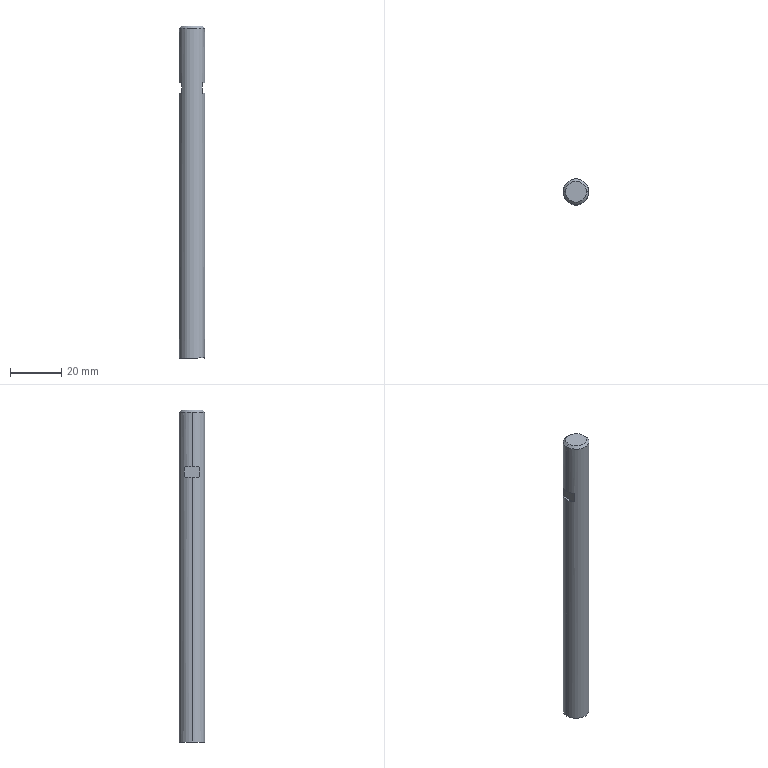Part | STEP file | fA_C85N25-100T(OUT) | 1 solid | 12 faces | box 10 x 10 x 129 mm | volume 10086 mm3 | plane 8 | cylinder 2 | cone 2 | commonest cylinder face diameters 10 x2
STEP:
#1=CARTESIAN_POINT('',(0.,0.,0.));
#2=DIRECTION('',(0.,0.,1.));
#3=DIRECTION('',(1.,0.,0.));
#4=AXIS2_PLACEMENT_3D('',#1,#2,#3);
#5=CARTESIAN_POINT('',(5.,0.,-1.));
#6=VERTEX_POINT('',#5);
#7=CARTESIAN_POINT('',(-5.,0.,-1.));
#8=VERTEX_POINT('',#7);
#9=CARTESIAN_POINT('',(0.,0.,-1.));
#10=DIRECTION('',(0.,0.,1.));
#11=DIRECTION('',(1.,0.,0.));
#12=AXIS2_PLACEMENT_3D('',#9,#10,#11);
#13=CIRCLE('',#12,5.);
#14=CARTESIAN_POINT('',(0.,0.,127.08));
#15=DIRECTION('',(0.,0.,1.));
#16=DIRECTION('',(1.,0.,0.));
#17=AXIS2_PLACEMENT_3D('',#14,#15,#16);
#18=CYLINDRICAL_SURFACE('',#17,5.);
#19=CARTESIAN_POINT('',(0.,-128.08));
#20=DIRECTION('',(1.,0.));
#21=VECTOR('',#20,1.);
#22=LINE('',#19,#21);
#23=(GEOMETRIC_REPRESENTATION_CONTEXT(2)PARAMETRIC_REPRESENTATION_CONTEXT()REPRESENTATION_CONTEXT('',''));
#24=DEFINITIONAL_REPRESENTATION('',(#22),#23);
#25=PCURVE('',#18,#24);
#26=CARTESIAN_POINT('',(5.06,5.,-1.));
#27=DIRECTION('',(0.,0.,-1.));
#28=DIRECTION('',(0.,1.,0.));
#29=AXIS2_PLACEMENT_3D('',#26,#27,#28);
#30=PLANE('',#29);
#31=CARTESIAN_POINT('',(-5.,-0.06));
#32=CARTESIAN_POINT('',(3.66,-0.06));
#33=CARTESIAN_POINT('',(-0.6699,-7.56));
#34=CARTESIAN_POINT('',(-5.,-15.06));
#35=CARTESIAN_POINT('',(-9.33,-7.56));
#36=CARTESIAN_POINT('',(-13.66,-0.06));
#37=CARTESIAN_POINT('',(-5.,-0.06));
#38=(BOUNDED_CURVE()B_SPLINE_CURVE(2,(#31,#32,#33,#34,#35,#36,#37),.UNSPECIFIED.,.T.,.F.)B_SPLINE_CURVE_WITH_KNOTS((1,2,2,2,2,1),(-2.094,0.,2.094,4.189,6.283,8.378),.UNSPECIFIED.)CURVE()GEOMETRIC_REPRESENTATION_ITEM()RATIONAL_B_SPLINE_CURVE((1.,0.5,1.,0.5,1.,0.5,1.))REPRESENTATION_ITEM(''));
#39=(GEOMETRIC_REPRESENTATION_CONTEXT(2)PARAMETRIC_REPRESENTATION_CONTEXT()REPRESENTATION_CONTEXT('',''));
#40=DEFINITIONAL_REPRESENTATION('',(#38),#39);
#41=PCURVE('',#30,#40);
#42=SURFACE_CURVE('',#13,(#25,#41),.PCURVE_S1.);
#43=EDGE_CURVE('',#6,#8,#42,.T.);
#44=ORIENTED_EDGE('',*,*,#43,.T.);
#45=CARTESIAN_POINT('',(-5.,0.,101.9));
#46=VERTEX_POINT('',#45);
#47=CARTESIAN_POINT('',(-5.,0.,127.08));
#48=DIRECTION('',(0.,0.,1.));
#49=VECTOR('',#48,1.);
#50=LINE('',#47,#49);
#51=CARTESIAN_POINT('',(3.142,0.));
#52=DIRECTION('',(0.,1.));
#53=VECTOR('',#52,1.);
#54=LINE('',#51,#53);
#55=(GEOMETRIC_REPRESENTATION_CONTEXT(2)PARAMETRIC_REPRESENTATION_CONTEXT()REPRESENTATION_CONTEXT('',''));
#56=DEFINITIONAL_REPRESENTATION('',(#54),#55);
#57=PCURVE('',#18,#56);
#58=CARTESIAN_POINT('',(0.,0.,127.08));
#59=DIRECTION('',(0.,0.,1.));
#60=DIRECTION('',(1.,0.,0.));
#61=AXIS2_PLACEMENT_3D('',#58,#59,#60);
#62=CYLINDRICAL_SURFACE('',#61,5.);
#63=CARTESIAN_POINT('',(3.142,0.));
#64=DIRECTION('',(0.,1.));
#65=VECTOR('',#64,1.);
#66=LINE('',#63,#65);
#67=(GEOMETRIC_REPRESENTATION_CONTEXT(2)PARAMETRIC_REPRESENTATION_CONTEXT()REPRESENTATION_CONTEXT('',''));
#68=DEFINITIONAL_REPRESENTATION('',(#66),#67);
#69=PCURVE('',#62,#68);
#70=SURFACE_CURVE('',#50,(#57,#69),.PCURVE_S1.);
#71=EDGE_CURVE('',#8,#46,#70,.T.);
#72=ORIENTED_EDGE('',*,*,#71,.T.);
#73=CARTESIAN_POINT('',(-4.,3.,101.9));
#74=VERTEX_POINT('',#73);
#75=CARTESIAN_POINT('',(0.,0.,101.9));
#76=DIRECTION('',(0.,0.,-1.));
#77=DIRECTION('',(1.,0.,0.));
#78=AXIS2_PLACEMENT_3D('',#75,#76,#77);
#79=CIRCLE('',#78,5.);
#80=CARTESIAN_POINT('',(6.283,-25.18));
#81=DIRECTION('',(-1.,0.));
#82=VECTOR('',#81,1.);
#83=LINE('',#80,#82);
#84=(GEOMETRIC_REPRESENTATION_CONTEXT(2)PARAMETRIC_REPRESENTATION_CONTEXT()REPRESENTATION_CONTEXT('',''));
#85=DEFINITIONAL_REPRESENTATION('',(#83),#84);
#86=PCURVE('',#18,#85);
#87=CARTESIAN_POINT('',(-5.006,-3.036,101.9));
#88=DIRECTION('',(0.,0.,1.));
#89=DIRECTION('',(1.,0.,0.));
#90=AXIS2_PLACEMENT_3D('',#87,#88,#89);
#91=PLANE('',#90);
#92=CARTESIAN_POINT('',(10.006,3.036));
#93=CARTESIAN_POINT('',(10.006,-5.624));
#94=CARTESIAN_POINT('',(2.506,-1.294));
#95=CARTESIAN_POINT('',(-4.994,3.036));
#96=CARTESIAN_POINT('',(2.506,7.366));
#97=CARTESIAN_POINT('',(10.006,11.696));
#98=CARTESIAN_POINT('',(10.006,3.036));
#99=(BOUNDED_CURVE()B_SPLINE_CURVE(2,(#92,#93,#94,#95,#96,#97,#98),.UNSPECIFIED.,.T.,.F.)B_SPLINE_CURVE_WITH_KNOTS((1,2,2,2,2,1),(-2.094,0.,2.094,4.189,6.283,8.378),.UNSPECIFIED.)CURVE()GEOMETRIC_REPRESENTATION_ITEM()RATIONAL_B_SPLINE_CURVE((1.,0.5,1.,0.5,1.,0.5,1.))REPRESENTATION_ITEM(''));
#100=(GEOMETRIC_REPRESENTATION_CONTEXT(2)PARAMETRIC_REPRESENTATION_CONTEXT()REPRESENTATION_CONTEXT('',''));
#101=DEFINITIONAL_REPRESENTATION('',(#99),#100);
#102=PCURVE('',#91,#101);
#103=SURFACE_CURVE('',#79,(#86,#102),.PCURVE_S1.);
#104=EDGE_CURVE('',#46,#74,#103,.T.);
#105=ORIENTED_EDGE('',*,*,#104,.T.);
#106=CARTESIAN_POINT('',(-4.,3.,105.9));
#107=VERTEX_POINT('',#106);
#108=CARTESIAN_POINT('',(-4.,3.,127.08));
#109=DIRECTION('',(0.,0.,1.));
#110=VECTOR('',#109,1.);
#111=LINE('',#108,#110);
#112=CARTESIAN_POINT('',(2.498,0.));
#113=DIRECTION('',(0.,1.));
#114=VECTOR('',#113,1.);
#115=LINE('',#112,#114);
#116=(GEOMETRIC_REPRESENTATION_CONTEXT(2)PARAMETRIC_REPRESENTATION_CONTEXT()REPRESENTATION_CONTEXT('',''));
#117=DEFINITIONAL_REPRESENTATION('',(#115),#116);
#118=PCURVE('',#18,#117);
#119=CARTESIAN_POINT('',(-4.,-3.,105.9));
#120=DIRECTION('',(-1.,0.,0.));
#121=DIRECTION('',(0.,0.,1.));
#122=AXIS2_PLACEMENT_3D('',#119,#120,#121);
#123=PLANE('',#122);
#124=CARTESIAN_POINT('',(21.18,6.));
#125=DIRECTION('',(1.,0.));
#126=VECTOR('',#125,1.);
#127=LINE('',#124,#126);
#128=(GEOMETRIC_REPRESENTATION_CONTEXT(2)PARAMETRIC_REPRESENTATION_CONTEXT()REPRESENTATION_CONTEXT('',''));
#129=DEFINITIONAL_REPRESENTATION('',(#127),#128);
#130=PCURVE('',#123,#129);
#131=SURFACE_CURVE('',#111,(#118,#130),.PCURVE_S1.);
#132=EDGE_CURVE('',#74,#107,#131,.T.);
#133=ORIENTED_EDGE('',*,*,#132,.T.);
#134=CARTESIAN_POINT('',(-5.,0.,105.9));
#135=VERTEX_POINT('',#134);
#136=CARTESIAN_POINT('',(0.,0.,105.9));
#137=DIRECTION('',(0.,0.,1.));
#138=DIRECTION('',(1.,0.,0.));
#139=AXIS2_PLACEMENT_3D('',#136,#137,#138);
#140=CIRCLE('',#139,5.);
#141=CARTESIAN_POINT('',(0.,-21.18));
#142=DIRECTION('',(1.,0.));
#143=VECTOR('',#142,1.);
#144=LINE('',#141,#143);
#145=(GEOMETRIC_REPRESENTATION_CONTEXT(2)PARAMETRIC_REPRESENTATION_CONTEXT()REPRESENTATION_CONTEXT('',''));
#146=DEFINITIONAL_REPRESENTATION('',(#144),#145);
#147=PCURVE('',#18,#146);
#148=CARTESIAN_POINT('',(-4.,-3.036,105.9));
#149=DIRECTION('',(0.,0.,-1.));
#150=DIRECTION('',(-1.,0.,0.));
#151=AXIS2_PLACEMENT_3D('',#148,#149,#150);
#152=PLANE('',#151);
#153=CARTESIAN_POINT('',(-9.,3.036));
#154=CARTESIAN_POINT('',(-9.,11.696));
#155=CARTESIAN_POINT('',(-1.5,7.366));
#156=CARTESIAN_POINT('',(6.,3.036));
#157=CARTESIAN_POINT('',(-1.5,-1.294));
#158=CARTESIAN_POINT('',(-9.,-5.624));
#159=CARTESIAN_POINT('',(-9.,3.036));
#160=(BOUNDED_CURVE()B_SPLINE_CURVE(2,(#153,#154,#155,#156,#157,#158,#159),.UNSPECIFIED.,.T.,.F.)B_SPLINE_CURVE_WITH_KNOTS((1,2,2,2,2,1),(-2.094,0.,2.094,4.189,6.283,8.378),.UNSPECIFIED.)CURVE()GEOMETRIC_REPRESENTATION_ITEM()RATIONAL_B_SPLINE_CURVE((1.,0.5,1.,0.5,1.,0.5,1.))REPRESENTATION_ITEM(''));
#161=(GEOMETRIC_REPRESENTATION_CONTEXT(2)PARAMETRIC_REPRESENTATION_CONTEXT()REPRESENTATION_CONTEXT('',''));
#162=DEFINITIONAL_REPRESENTATION('',(#160),#161);
#163=PCURVE('',#152,#162);
#164=SURFACE_CURVE('',#140,(#147,#163),.PCURVE_S1.);
#165=EDGE_CURVE('',#107,#135,#164,.T.);
#166=ORIENTED_EDGE('',*,*,#165,.T.);
#167=CARTESIAN_POINT('',(-5.,0.,127.08));
#168=VERTEX_POINT('',#167);
#169=CARTESIAN_POINT('',(-5.,0.,127.08));
#170=DIRECTION('',(0.,0.,1.));
#171=VECTOR('',#170,1.);
#172=LINE('',#169,#171);
#173=CARTESIAN_POINT('',(3.142,0.));
#174=DIRECTION('',(0.,1.));
#175=VECTOR('',#174,1.);
#176=LINE('',#173,#175);
#177=(GEOMETRIC_REPRESENTATION_CONTEXT(2)PARAMETRIC_REPRESENTATION_CONTEXT()REPRESENTATION_CONTEXT('',''));
#178=DEFINITIONAL_REPRESENTATION('',(#176),#177);
#179=PCURVE('',#18,#178);
#180=CARTESIAN_POINT('',(3.142,0.));
#181=DIRECTION('',(0.,1.));
#182=VECTOR('',#181,1.);
#183=LINE('',#180,#182);
#184=(GEOMETRIC_REPRESENTATION_CONTEXT(2)PARAMETRIC_REPRESENTATION_CONTEXT()REPRESENTATION_CONTEXT('',''));
#185=DEFINITIONAL_REPRESENTATION('',(#183),#184);
#186=PCURVE('',#62,#185);
#187=SURFACE_CURVE('',#172,(#179,#186),.PCURVE_S1.);
#188=EDGE_CURVE('',#135,#168,#187,.T.);
#189=ORIENTED_EDGE('',*,*,#188,.T.);
#190=CARTESIAN_POINT('',(5.,0.,127.08));
#191=VERTEX_POINT('',#190);
#192=CARTESIAN_POINT('',(0.,0.,127.08));
#193=DIRECTION('',(0.,0.,-1.));
#194=DIRECTION('',(1.,0.,0.));
#195=AXIS2_PLACEMENT_3D('',#192,#193,#194);
#196=CIRCLE('',#195,5.);
#197=CARTESIAN_POINT('',(6.283,0.));
#198=DIRECTION('',(-1.,0.));
#199=VECTOR('',#198,1.);
#200=LINE('',#197,#199);
#201=(GEOMETRIC_REPRESENTATION_CONTEXT(2)PARAMETRIC_REPRESENTATION_CONTEXT()REPRESENTATION_CONTEXT('',''));
#202=DEFINITIONAL_REPRESENTATION('',(#200),#201);
#203=PCURVE('',#18,#202);
#204=CARTESIAN_POINT('',(0.,0.,127.08));
#205=DIRECTION('',(0.,0.,-1.));
#206=DIRECTION('',(-1.,0.,0.));
#207=AXIS2_PLACEMENT_3D('',#204,#205,#206);
#208=CONICAL_SURFACE('',#207,5.,0.7854);
#209=CARTESIAN_POINT('',(-3.142,0.));
#210=DIRECTION('',(1.,0.));
#211=VECTOR('',#210,1.);
#212=LINE('',#209,#211);
#213=(GEOMETRIC_REPRESENTATION_CONTEXT(2)PARAMETRIC_REPRESENTATION_CONTEXT()REPRESENTATION_CONTEXT('',''));
#214=DEFINITIONAL_REPRESENTATION('',(#212),#213);
#215=PCURVE('',#208,#214);
#216=SURFACE_CURVE('',#196,(#203,#215),.PCURVE_S1.);
#217=EDGE_CURVE('',#168,#191,#216,.T.);
#218=ORIENTED_EDGE('',*,*,#217,.T.);
#219=CARTESIAN_POINT('',(5.,0.,105.9));
#220=VERTEX_POINT('',#219);
#221=CARTESIAN_POINT('',(5.,0.,127.08));
#222=DIRECTION('',(0.,0.,1.));
#223=VECTOR('',#222,1.);
#224=LINE('',#221,#223);
#225=CARTESIAN_POINT('',(0.,0.));
#226=DIRECTION('',(0.,1.));
#227=VECTOR('',#226,1.);
#228=LINE('',#225,#227);
#229=(GEOMETRIC_REPRESENTATION_CONTEXT(2)PARAMETRIC_REPRESENTATION_CONTEXT()REPRESENTATION_CONTEXT('',''));
#230=DEFINITIONAL_REPRESENTATION('',(#228),#229);
#231=PCURVE('',#18,#230);
#232=CARTESIAN_POINT('',(6.283,0.));
#233=DIRECTION('',(0.,1.));
#234=VECTOR('',#233,1.);
#235=LINE('',#232,#234);
#236=(GEOMETRIC_REPRESENTATION_CONTEXT(2)PARAMETRIC_REPRESENTATION_CONTEXT()REPRESENTATION_CONTEXT('',''));
#237=DEFINITIONAL_REPRESENTATION('',(#235),#236);
#238=PCURVE('',#62,#237);
#239=SURFACE_CURVE('',#224,(#231,#238),.PCURVE_S1.);
#240=EDGE_CURVE('',#220,#191,#239,.T.);
#241=ORIENTED_EDGE('',*,*,#240,.F.);
#242=CARTESIAN_POINT('',(4.,3.,105.9));
#243=VERTEX_POINT('',#242);
#244=CARTESIAN_POINT('',(0.,0.,105.9));
#245=DIRECTION('',(0.,0.,1.));
#246=DIRECTION('',(1.,0.,0.));
#247=AXIS2_PLACEMENT_3D('',#244,#245,#246);
#248=CIRCLE('',#247,5.);
#249=CARTESIAN_POINT('',(0.,-21.18));
#250=DIRECTION('',(1.,0.));
#251=VECTOR('',#250,1.);
#252=LINE('',#249,#251);
#253=(GEOMETRIC_REPRESENTATION_CONTEXT(2)PARAMETRIC_REPRESENTATION_CONTEXT()REPRESENTATION_CONTEXT('',''));
#254=DEFINITIONAL_REPRESENTATION('',(#252),#253);
#255=PCURVE('',#18,#254);
#256=CARTESIAN_POINT('',(5.006,-3.036,105.9));
#257=DIRECTION('',(0.,0.,-1.));
#258=DIRECTION('',(-1.,0.,0.));
#259=AXIS2_PLACEMENT_3D('',#256,#257,#258);
#260=PLANE('',#259);
#261=CARTESIAN_POINT('',(0.006,3.036));
#262=CARTESIAN_POINT('',(0.006,11.696));
#263=CARTESIAN_POINT('',(7.506,7.366));
#264=CARTESIAN_POINT('',(15.006,3.036));
#265=CARTESIAN_POINT('',(7.506,-1.294));
#266=CARTESIAN_POINT('',(0.006,-5.624));
#267=CARTESIAN_POINT('',(0.006,3.036));
#268=(BOUNDED_CURVE()B_SPLINE_CURVE(2,(#261,#262,#263,#264,#265,#266,#267),.UNSPECIFIED.,.T.,.F.)B_SPLINE_CURVE_WITH_KNOTS((1,2,2,2,2,1),(-2.094,0.,2.094,4.189,6.283,8.378),.UNSPECIFIED.)CURVE()GEOMETRIC_REPRESENTATION_ITEM()RATIONAL_B_SPLINE_CURVE((1.,0.5,1.,0.5,1.,0.5,1.))REPRESENTATION_ITEM(''));
#269=(GEOMETRIC_REPRESENTATION_CONTEXT(2)PARAMETRIC_REPRESENTATION_CONTEXT()REPRESENTATION_CONTEXT('',''));
#270=DEFINITIONAL_REPRESENTATION('',(#268),#269);
#271=PCURVE('',#260,#270);
#272=SURFACE_CURVE('',#248,(#255,#271),.PCURVE_S1.);
#273=EDGE_CURVE('',#220,#243,#272,.T.);
#274=ORIENTED_EDGE('',*,*,#273,.T.);
#275=CARTESIAN_POINT('',(4.,3.,101.9));
#276=VERTEX_POINT('',#275);
#277=CARTESIAN_POINT('',(4.,3.,127.08));
#278=DIRECTION('',(0.,0.,-1.));
#279=VECTOR('',#278,1.);
#280=LINE('',#277,#279);
#281=CARTESIAN_POINT('',(0.6435,0.));
#282=DIRECTION('',(0.,-1.));
#283=VECTOR('',#282,1.);
#284=LINE('',#281,#283);
#285=(GEOMETRIC_REPRESENTATION_CONTEXT(2)PARAMETRIC_REPRESENTATION_CONTEXT()REPRESENTATION_CONTEXT('',''));
#286=DEFINITIONAL_REPRESENTATION('',(#284),#285);
#287=PCURVE('',#18,#286);
#288=CARTESIAN_POINT('',(4.,3.,105.9));
#289=DIRECTION('',(1.,0.,0.));
#290=DIRECTION('',(0.,0.,-1.));
#291=AXIS2_PLACEMENT_3D('',#288,#289,#290);
#292=PLANE('',#291);
#293=CARTESIAN_POINT('',(-21.18,0.));
#294=DIRECTION('',(1.,0.));
#295=VECTOR('',#294,1.);
#296=LINE('',#293,#295);
#297=(GEOMETRIC_REPRESENTATION_CONTEXT(2)PARAMETRIC_REPRESENTATION_CONTEXT()REPRESENTATION_CONTEXT('',''));
#298=DEFINITIONAL_REPRESENTATION('',(#296),#297);
#299=PCURVE('',#292,#298);
#300=SURFACE_CURVE('',#280,(#287,#299),.PCURVE_S1.);
#301=EDGE_CURVE('',#243,#276,#300,.T.);
#302=ORIENTED_EDGE('',*,*,#301,.T.);
#303=CARTESIAN_POINT('',(5.,0.,101.9));
#304=VERTEX_POINT('',#303);
#305=CARTESIAN_POINT('',(0.,0.,101.9));
#306=DIRECTION('',(0.,0.,-1.));
#307=DIRECTION('',(1.,0.,0.));
#308=AXIS2_PLACEMENT_3D('',#305,#306,#307);
#309=CIRCLE('',#308,5.);
#310=CARTESIAN_POINT('',(6.283,-25.18));
#311=DIRECTION('',(-1.,0.));
#312=VECTOR('',#311,1.);
#313=LINE('',#310,#312);
#314=(GEOMETRIC_REPRESENTATION_CONTEXT(2)PARAMETRIC_REPRESENTATION_CONTEXT()REPRESENTATION_CONTEXT('',''));
#315=DEFINITIONAL_REPRESENTATION('',(#313),#314);
#316=PCURVE('',#18,#315);
#317=CARTESIAN_POINT('',(4.,-3.036,101.9));
#318=DIRECTION('',(0.,0.,1.));
#319=DIRECTION('',(1.,0.,0.));
#320=AXIS2_PLACEMENT_3D('',#317,#318,#319);
#321=PLANE('',#320);
#322=CARTESIAN_POINT('',(1.,3.036));
#323=CARTESIAN_POINT('',(1.,-5.624));
#324=CARTESIAN_POINT('',(-6.5,-1.294));
#325=CARTESIAN_POINT('',(-14.,3.036));
#326=CARTESIAN_POINT('',(-6.5,7.366));
#327=CARTESIAN_POINT('',(1.,11.696));
#328=CARTESIAN_POINT('',(1.,3.036));
#329=(BOUNDED_CURVE()B_SPLINE_CURVE(2,(#322,#323,#324,#325,#326,#327,#328),.UNSPECIFIED.,.T.,.F.)B_SPLINE_CURVE_WITH_KNOTS((1,2,2,2,2,1),(-2.094,0.,2.094,4.189,6.283,8.378),.UNSPECIFIED.)CURVE()GEOMETRIC_REPRESENTATION_ITEM()RATIONAL_B_SPLINE_CURVE((1.,0.5,1.,0.5,1.,0.5,1.))REPRESENTATION_ITEM(''));
#330=(GEOMETRIC_REPRESENTATION_CONTEXT(2)PARAMETRIC_REPRESENTATION_CONTEXT()REPRESENTATION_CONTEXT('',''));
#331=DEFINITIONAL_REPRESENTATION('',(#329),#330);
#332=PCURVE('',#321,#331);
#333=SURFACE_CURVE('',#309,(#316,#332),.PCURVE_S1.);
#334=EDGE_CURVE('',#276,#304,#333,.T.);
#335=ORIENTED_EDGE('',*,*,#334,.T.);
#336=CARTESIAN_POINT('',(5.,0.,127.08));
#337=DIRECTION('',(0.,0.,1.));
#338=VECTOR('',#337,1.);
#339=LINE('',#336,#338);
#340=CARTESIAN_POINT('',(0.,0.));
#341=DIRECTION('',(0.,1.));
#342=VECTOR('',#341,1.);
#343=LINE('',#340,#342);
#344=(GEOMETRIC_REPRESENTATION_CONTEXT(2)PARAMETRIC_REPRESENTATION_CONTEXT()REPRESENTATION_CONTEXT('',''));
#345=DEFINITIONAL_REPRESENTATION('',(#343),#344);
#346=PCURVE('',#18,#345);
#347=CARTESIAN_POINT('',(6.283,0.));
#348=DIRECTION('',(0.,1.));
#349=VECTOR('',#348,1.);
#350=LINE('',#347,#349);
#351=(GEOMETRIC_REPRESENTATION_CONTEXT(2)PARAMETRIC_REPRESENTATION_CONTEXT()REPRESENTATION_CONTEXT('',''));
#352=DEFINITIONAL_REPRESENTATION('',(#350),#351);
#353=PCURVE('',#62,#352);
#354=SURFACE_CURVE('',#339,(#346,#353),.PCURVE_S1.);
#355=EDGE_CURVE('',#6,#304,#354,.T.);
#356=ORIENTED_EDGE('',*,*,#355,.F.);
#357=EDGE_LOOP('',(#44,#72,#105,#133,#166,#189,#218,#241,#274,#302,#335,#356));
#358=FACE_BOUND('',#357,.T.);
#359=ADVANCED_FACE('',(#358),#18,.T.);
#360=CARTESIAN_POINT('',(-4.08,0.,128.));
#361=VERTEX_POINT('',#360);
#362=CARTESIAN_POINT('',(4.08,0.,128.));
#363=VERTEX_POINT('',#362);
#364=CARTESIAN_POINT('',(0.,0.,128.));
#365=DIRECTION('',(0.,0.,-1.));
#366=DIRECTION('',(-1.,0.,0.));
#367=AXIS2_PLACEMENT_3D('',#364,#365,#366);
#368=CIRCLE('',#367,4.08);
#369=CARTESIAN_POINT('',(0.,-0.92));
#370=DIRECTION('',(1.,0.));
#371=VECTOR('',#370,1.);
#372=LINE('',#369,#371);
#373=(GEOMETRIC_REPRESENTATION_CONTEXT(2)PARAMETRIC_REPRESENTATION_CONTEXT()REPRESENTATION_CONTEXT('',''));
#374=DEFINITIONAL_REPRESENTATION('',(#372),#373);
#375=PCURVE('',#208,#374);
#376=CARTESIAN_POINT('',(4.129,-4.08,128.));
#377=DIRECTION('',(0.,0.,1.));
#378=DIRECTION('',(1.,0.,0.));
#379=AXIS2_PLACEMENT_3D('',#376,#377,#378);
#380=PLANE('',#379);
#381=CARTESIAN_POINT('',(-8.209,4.08));
#382=CARTESIAN_POINT('',(-8.209,11.147));
#383=CARTESIAN_POINT('',(-2.089,7.613));
#384=CARTESIAN_POINT('',(4.031,4.08));
#385=CARTESIAN_POINT('',(-2.089,0.5466));
#386=CARTESIAN_POINT('',(-8.209,-2.987));
#387=CARTESIAN_POINT('',(-8.209,4.08));
#388=(BOUNDED_CURVE()B_SPLINE_CURVE(2,(#381,#382,#383,#384,#385,#386,#387),.UNSPECIFIED.,.T.,.F.)B_SPLINE_CURVE_WITH_KNOTS((1,2,2,2,2,1),(-2.094,0.,2.094,4.189,6.283,8.378),.UNSPECIFIED.)CURVE()GEOMETRIC_REPRESENTATION_ITEM()RATIONAL_B_SPLINE_CURVE((1.,0.5,1.,0.5,1.,0.5,1.))REPRESENTATION_ITEM(''));
#389=(GEOMETRIC_REPRESENTATION_CONTEXT(2)PARAMETRIC_REPRESENTATION_CONTEXT()REPRESENTATION_CONTEXT('',''));
#390=DEFINITIONAL_REPRESENTATION('',(#388),#389);
#391=PCURVE('',#380,#390);
#392=SURFACE_CURVE('',#368,(#375,#391),.PCURVE_S1.);
#393=EDGE_CURVE('',#361,#363,#392,.T.);
#394=ORIENTED_EDGE('',*,*,#393,.T.);
#395=CARTESIAN_POINT('',(5.,0.,127.08));
#396=DIRECTION('',(0.7071,0.,-0.7071));
#397=VECTOR('',#396,1.);
#398=LINE('',#395,#397);
#399=CARTESIAN_POINT('',(3.142,0.));
#400=DIRECTION('',(0.,1.));
#401=VECTOR('',#400,1.);
#402=LINE('',#399,#401);
#403=(GEOMETRIC_REPRESENTATION_CONTEXT(2)PARAMETRIC_REPRESENTATION_CONTEXT()REPRESENTATION_CONTEXT('',''));
#404=DEFINITIONAL_REPRESENTATION('',(#402),#403);
#405=PCURVE('',#208,#404);
#406=CARTESIAN_POINT('',(0.,0.,127.08));
#407=DIRECTION('',(0.,0.,-1.));
#408=DIRECTION('',(-1.,0.,0.));
#409=AXIS2_PLACEMENT_3D('',#406,#407,#408);
#410=CONICAL_SURFACE('',#409,5.,0.7854);
#411=CARTESIAN_POINT('',(3.142,0.));
#412=DIRECTION('',(0.,1.));
#413=VECTOR('',#412,1.);
#414=LINE('',#411,#413);
#415=(GEOMETRIC_REPRESENTATION_CONTEXT(2)PARAMETRIC_REPRESENTATION_CONTEXT()REPRESENTATION_CONTEXT('',''));
#416=DEFINITIONAL_REPRESENTATION('',(#414),#415);
#417=PCURVE('',#410,#416);
#418=SURFACE_CURVE('',#398,(#405,#417),.PCURVE_S1.);
#419=EDGE_CURVE('',#363,#191,#418,.T.);
#420=ORIENTED_EDGE('',*,*,#419,.T.);
#421=ORIENTED_EDGE('',*,*,#217,.F.);
#422=CARTESIAN_POINT('',(-5.,0.,127.08));
#423=DIRECTION('',(-0.7071,0.,-0.7071));
#424=VECTOR('',#423,1.);
#425=LINE('',#422,#424);
#426=CARTESIAN_POINT('',(0.,0.));
#427=DIRECTION('',(0.,1.));
#428=VECTOR('',#427,1.);
#429=LINE('',#426,#428);
#430=(GEOMETRIC_REPRESENTATION_CONTEXT(2)PARAMETRIC_REPRESENTATION_CONTEXT()REPRESENTATION_CONTEXT('',''));
#431=DEFINITIONAL_REPRESENTATION('',(#429),#430);
#432=PCURVE('',#208,#431);
#433=CARTESIAN_POINT('',(6.283,0.));
#434=DIRECTION('',(0.,1.));
#435=VECTOR('',#434,1.);
#436=LINE('',#433,#435);
#437=(GEOMETRIC_REPRESENTATION_CONTEXT(2)PARAMETRIC_REPRESENTATION_CONTEXT()REPRESENTATION_CONTEXT('',''));
#438=DEFINITIONAL_REPRESENTATION('',(#436),#437);
#439=PCURVE('',#410,#438);
#440=SURFACE_CURVE('',#425,(#432,#439),.PCURVE_S1.);
#441=EDGE_CURVE('',#361,#168,#440,.T.);
#442=ORIENTED_EDGE('',*,*,#441,.F.);
#443=EDGE_LOOP('',(#394,#420,#421,#442));
#444=FACE_BOUND('',#443,.T.);
#445=ADVANCED_FACE('',(#444),#208,.T.);
#446=ORIENTED_EDGE('',*,*,#71,.F.);
#447=CARTESIAN_POINT('',(0.,0.,-1.));
#448=DIRECTION('',(0.,0.,1.));
#449=DIRECTION('',(1.,0.,0.));
#450=AXIS2_PLACEMENT_3D('',#447,#448,#449);
#451=CIRCLE('',#450,5.);
#452=CARTESIAN_POINT('',(0.,-128.08));
#453=DIRECTION('',(1.,0.));
#454=VECTOR('',#453,1.);
#455=LINE('',#452,#454);
#456=(GEOMETRIC_REPRESENTATION_CONTEXT(2)PARAMETRIC_REPRESENTATION_CONTEXT()REPRESENTATION_CONTEXT('',''));
#457=DEFINITIONAL_REPRESENTATION('',(#455),#456);
#458=PCURVE('',#62,#457);
#459=CARTESIAN_POINT('',(-5.,-0.06));
#460=CARTESIAN_POINT('',(3.66,-0.06));
#461=CARTESIAN_POINT('',(-0.6699,-7.56));
#462=CARTESIAN_POINT('',(-5.,-15.06));
#463=CARTESIAN_POINT('',(-9.33,-7.56));
#464=CARTESIAN_POINT('',(-13.66,-0.06));
#465=CARTESIAN_POINT('',(-5.,-0.06));
#466=(BOUNDED_CURVE()B_SPLINE_CURVE(2,(#459,#460,#461,#462,#463,#464,#465),.UNSPECIFIED.,.T.,.F.)B_SPLINE_CURVE_WITH_KNOTS((1,2,2,2,2,1),(-2.094,0.,2.094,4.189,6.283,8.378),.UNSPECIFIED.)CURVE()GEOMETRIC_REPRESENTATION_ITEM()RATIONAL_B_SPLINE_CURVE((1.,0.5,1.,0.5,1.,0.5,1.))REPRESENTATION_ITEM(''));
#467=(GEOMETRIC_REPRESENTATION_CONTEXT(2)PARAMETRIC_REPRESENTATION_CONTEXT()REPRESENTATION_CONTEXT('',''));
#468=DEFINITIONAL_REPRESENTATION('',(#466),#467);
#469=PCURVE('',#30,#468);
#470=SURFACE_CURVE('',#451,(#458,#469),.PCURVE_S1.);
#471=EDGE_CURVE('',#8,#6,#470,.T.);
#472=ORIENTED_EDGE('',*,*,#471,.T.);
#473=ORIENTED_EDGE('',*,*,#355,.T.);
#474=CARTESIAN_POINT('',(4.,-3.,101.9));
#475=VERTEX_POINT('',#474);
#476=CARTESIAN_POINT('',(0.,0.,101.9));
#477=DIRECTION('',(0.,0.,-1.));
#478=DIRECTION('',(1.,0.,0.));
#479=AXIS2_PLACEMENT_3D('',#476,#477,#478);
#480=CIRCLE('',#479,5.);
#481=CARTESIAN_POINT('',(6.283,-25.18));
#482=DIRECTION('',(-1.,0.));
#483=VECTOR('',#482,1.);
#484=LINE('',#481,#483);
#485=(GEOMETRIC_REPRESENTATION_CONTEXT(2)PARAMETRIC_REPRESENTATION_CONTEXT()REPRESENTATION_CONTEXT('',''));
#486=DEFINITIONAL_REPRESENTATION('',(#484),#485);
#487=PCURVE('',#62,#486);
#488=CARTESIAN_POINT('',(1.,3.036));
#489=CARTESIAN_POINT('',(1.,-5.624));
#490=CARTESIAN_POINT('',(-6.5,-1.294));
#491=CARTESIAN_POINT('',(-14.,3.036));
#492=CARTESIAN_POINT('',(-6.5,7.366));
#493=CARTESIAN_POINT('',(1.,11.696));
#494=CARTESIAN_POINT('',(1.,3.036));
#495=(BOUNDED_CURVE()B_SPLINE_CURVE(2,(#488,#489,#490,#491,#492,#493,#494),.UNSPECIFIED.,.T.,.F.)B_SPLINE_CURVE_WITH_KNOTS((1,2,2,2,2,1),(-2.094,0.,2.094,4.189,6.283,8.378),.UNSPECIFIED.)CURVE()GEOMETRIC_REPRESENTATION_ITEM()RATIONAL_B_SPLINE_CURVE((1.,0.5,1.,0.5,1.,0.5,1.))REPRESENTATION_ITEM(''));
#496=(GEOMETRIC_REPRESENTATION_CONTEXT(2)PARAMETRIC_REPRESENTATION_CONTEXT()REPRESENTATION_CONTEXT('',''));
#497=DEFINITIONAL_REPRESENTATION('',(#495),#496);
#498=PCURVE('',#321,#497);
#499=SURFACE_CURVE('',#480,(#487,#498),.PCURVE_S1.);
#500=EDGE_CURVE('',#304,#475,#499,.T.);
#501=ORIENTED_EDGE('',*,*,#500,.T.);
#502=CARTESIAN_POINT('',(4.,-3.,105.9));
#503=VERTEX_POINT('',#502);
#504=CARTESIAN_POINT('',(4.,-3.,127.08));
#505=DIRECTION('',(0.,0.,1.));
#506=VECTOR('',#505,1.);
#507=LINE('',#504,#506);
#508=CARTESIAN_POINT('',(5.64,0.));
#509=DIRECTION('',(0.,1.));
#510=VECTOR('',#509,1.);
#511=LINE('',#508,#510);
#512=(GEOMETRIC_REPRESENTATION_CONTEXT(2)PARAMETRIC_REPRESENTATION_CONTEXT()REPRESENTATION_CONTEXT('',''));
#513=DEFINITIONAL_REPRESENTATION('',(#511),#512);
#514=PCURVE('',#62,#513);
#515=CARTESIAN_POINT('',(-21.18,-6.));
#516=DIRECTION('',(-1.,0.));
#517=VECTOR('',#516,1.);
#518=LINE('',#515,#517);
#519=(GEOMETRIC_REPRESENTATION_CONTEXT(2)PARAMETRIC_REPRESENTATION_CONTEXT()REPRESENTATION_CONTEXT('',''));
#520=DEFINITIONAL_REPRESENTATION('',(#518),#519);
#521=PCURVE('',#292,#520);
#522=SURFACE_CURVE('',#507,(#514,#521),.PCURVE_S1.);
#523=EDGE_CURVE('',#475,#503,#522,.T.);
#524=ORIENTED_EDGE('',*,*,#523,.T.);
#525=CARTESIAN_POINT('',(0.,0.,105.9));
#526=DIRECTION('',(0.,0.,1.));
#527=DIRECTION('',(1.,0.,0.));
#528=AXIS2_PLACEMENT_3D('',#525,#526,#527);
#529=CIRCLE('',#528,5.);
#530=CARTESIAN_POINT('',(0.,-21.18));
#531=DIRECTION('',(1.,0.));
#532=VECTOR('',#531,1.);
#533=LINE('',#530,#532);
#534=(GEOMETRIC_REPRESENTATION_CONTEXT(2)PARAMETRIC_REPRESENTATION_CONTEXT()REPRESENTATION_CONTEXT('',''));
#535=DEFINITIONAL_REPRESENTATION('',(#533),#534);
#536=PCURVE('',#62,#535);
#537=CARTESIAN_POINT('',(0.006,3.036));
#538=CARTESIAN_POINT('',(0.006,11.696));
#539=CARTESIAN_POINT('',(7.506,7.366));
#540=CARTESIAN_POINT('',(15.006,3.036));
#541=CARTESIAN_POINT('',(7.506,-1.294));
#542=CARTESIAN_POINT('',(0.006,-5.624));
#543=CARTESIAN_POINT('',(0.006,3.036));
#544=(BOUNDED_CURVE()B_SPLINE_CURVE(2,(#537,#538,#539,#540,#541,#542,#543),.UNSPECIFIED.,.T.,.F.)B_SPLINE_CURVE_WITH_KNOTS((1,2,2,2,2,1),(-2.094,0.,2.094,4.189,6.283,8.378),.UNSPECIFIED.)CURVE()GEOMETRIC_REPRESENTATION_ITEM()RATIONAL_B_SPLINE_CURVE((1.,0.5,1.,0.5,1.,0.5,1.))REPRESENTATION_ITEM(''));
#545=(GEOMETRIC_REPRESENTATION_CONTEXT(2)PARAMETRIC_REPRESENTATION_CONTEXT()REPRESENTATION_CONTEXT('',''));
#546=DEFINITIONAL_REPRESENTATION('',(#544),#545);
#547=PCURVE('',#260,#546);
#548=SURFACE_CURVE('',#529,(#536,#547),.PCURVE_S1.);
#549=EDGE_CURVE('',#503,#220,#548,.T.);
#550=ORIENTED_EDGE('',*,*,#549,.T.);
#551=ORIENTED_EDGE('',*,*,#240,.T.);
#552=CARTESIAN_POINT('',(0.,0.,127.08));
#553=DIRECTION('',(0.,0.,-1.));
#554=DIRECTION('',(1.,0.,0.));
#555=AXIS2_PLACEMENT_3D('',#552,#553,#554);
#556=CIRCLE('',#555,5.);
#557=CARTESIAN_POINT('',(6.283,0.));
#558=DIRECTION('',(-1.,0.));
#559=VECTOR('',#558,1.);
#560=LINE('',#557,#559);
#561=(GEOMETRIC_REPRESENTATION_CONTEXT(2)PARAMETRIC_REPRESENTATION_CONTEXT()REPRESENTATION_CONTEXT('',''));
#562=DEFINITIONAL_REPRESENTATION('',(#560),#561);
#563=PCURVE('',#62,#562);
#564=CARTESIAN_POINT('',(3.142,0.));
#565=DIRECTION('',(1.,0.));
#566=VECTOR('',#565,1.);
#567=LINE('',#564,#566);
#568=(GEOMETRIC_REPRESENTATION_CONTEXT(2)PARAMETRIC_REPRESENTATION_CONTEXT()REPRESENTATION_CONTEXT('',''));
#569=DEFINITIONAL_REPRESENTATION('',(#567),#568);
#570=PCURVE('',#410,#569);
#571=SURFACE_CURVE('',#556,(#563,#570),.PCURVE_S1.);
#572=EDGE_CURVE('',#191,#168,#571,.T.);
#573=ORIENTED_EDGE('',*,*,#572,.T.);
#574=ORIENTED_EDGE('',*,*,#188,.F.);
#575=CARTESIAN_POINT('',(-4.,-3.,105.9));
#576=VERTEX_POINT('',#575);
#577=CARTESIAN_POINT('',(0.,0.,105.9));
#578=DIRECTION('',(0.,0.,1.));
#579=DIRECTION('',(1.,0.,0.));
#580=AXIS2_PLACEMENT_3D('',#577,#578,#579);
#581=CIRCLE('',#580,5.);
#582=CARTESIAN_POINT('',(0.,-21.18));
#583=DIRECTION('',(1.,0.));
#584=VECTOR('',#583,1.);
#585=LINE('',#582,#584);
#586=(GEOMETRIC_REPRESENTATION_CONTEXT(2)PARAMETRIC_REPRESENTATION_CONTEXT()REPRESENTATION_CONTEXT('',''));
#587=DEFINITIONAL_REPRESENTATION('',(#585),#586);
#588=PCURVE('',#62,#587);
#589=CARTESIAN_POINT('',(-9.,3.036));
#590=CARTESIAN_POINT('',(-9.,11.696));
#591=CARTESIAN_POINT('',(-1.5,7.366));
#592=CARTESIAN_POINT('',(6.,3.036));
#593=CARTESIAN_POINT('',(-1.5,-1.294));
#594=CARTESIAN_POINT('',(-9.,-5.624));
#595=CARTESIAN_POINT('',(-9.,3.036));
#596=(BOUNDED_CURVE()B_SPLINE_CURVE(2,(#589,#590,#591,#592,#593,#594,#595),.UNSPECIFIED.,.T.,.F.)B_SPLINE_CURVE_WITH_KNOTS((1,2,2,2,2,1),(-2.094,0.,2.094,4.189,6.283,8.378),.UNSPECIFIED.)CURVE()GEOMETRIC_REPRESENTATION_ITEM()RATIONAL_B_SPLINE_CURVE((1.,0.5,1.,0.5,1.,0.5,1.))REPRESENTATION_ITEM(''));
#597=(GEOMETRIC_REPRESENTATION_CONTEXT(2)PARAMETRIC_REPRESENTATION_CONTEXT()REPRESENTATION_CONTEXT('',''));
#598=DEFINITIONAL_REPRESENTATION('',(#596),#597);
#599=PCURVE('',#152,#598);
#600=SURFACE_CURVE('',#581,(#588,#599),.PCURVE_S1.);
#601=EDGE_CURVE('',#135,#576,#600,.T.);
#602=ORIENTED_EDGE('',*,*,#601,.T.);
#603=CARTESIAN_POINT('',(-4.,-3.,101.9));
#604=VERTEX_POINT('',#603);
#605=CARTESIAN_POINT('',(-4.,-3.,127.08));
#606=DIRECTION('',(0.,0.,-1.));
#607=VECTOR('',#606,1.);
#608=LINE('',#605,#607);
#609=CARTESIAN_POINT('',(3.785,0.));
#610=DIRECTION('',(0.,-1.));
#611=VECTOR('',#610,1.);
#612=LINE('',#609,#611);
#613=(GEOMETRIC_REPRESENTATION_CONTEXT(2)PARAMETRIC_REPRESENTATION_CONTEXT()REPRESENTATION_CONTEXT('',''));
#614=DEFINITIONAL_REPRESENTATION('',(#612),#613);
#615=PCURVE('',#62,#614);
#616=CARTESIAN_POINT('',(21.18,0.));
#617=DIRECTION('',(-1.,0.));
#618=VECTOR('',#617,1.);
#619=LINE('',#616,#618);
#620=(GEOMETRIC_REPRESENTATION_CONTEXT(2)PARAMETRIC_REPRESENTATION_CONTEXT()REPRESENTATION_CONTEXT('',''));
#621=DEFINITIONAL_REPRESENTATION('',(#619),#620);
#622=PCURVE('',#123,#621);
#623=SURFACE_CURVE('',#608,(#615,#622),.PCURVE_S1.);
#624=EDGE_CURVE('',#576,#604,#623,.T.);
#625=ORIENTED_EDGE('',*,*,#624,.T.);
#626=CARTESIAN_POINT('',(0.,0.,101.9));
#627=DIRECTION('',(0.,0.,-1.));
#628=DIRECTION('',(1.,0.,0.));
#629=AXIS2_PLACEMENT_3D('',#626,#627,#628);
#630=CIRCLE('',#629,5.);
#631=CARTESIAN_POINT('',(6.283,-25.18));
#632=DIRECTION('',(-1.,0.));
#633=VECTOR('',#632,1.);
#634=LINE('',#631,#633);
#635=(GEOMETRIC_REPRESENTATION_CONTEXT(2)PARAMETRIC_REPRESENTATION_CONTEXT()REPRESENTATION_CONTEXT('',''));
#636=DEFINITIONAL_REPRESENTATION('',(#634),#635);
#637=PCURVE('',#62,#636);
#638=CARTESIAN_POINT('',(10.006,3.036));
#639=CARTESIAN_POINT('',(10.006,-5.624));
#640=CARTESIAN_POINT('',(2.506,-1.294));
#641=CARTESIAN_POINT('',(-4.994,3.036));
#642=CARTESIAN_POINT('',(2.506,7.366));
#643=CARTESIAN_POINT('',(10.006,11.696));
#644=CARTESIAN_POINT('',(10.006,3.036));
#645=(BOUNDED_CURVE()B_SPLINE_CURVE(2,(#638,#639,#640,#641,#642,#643,#644),.UNSPECIFIED.,.T.,.F.)B_SPLINE_CURVE_WITH_KNOTS((1,2,2,2,2,1),(-2.094,0.,2.094,4.189,6.283,8.378),.UNSPECIFIED.)CURVE()GEOMETRIC_REPRESENTATION_ITEM()RATIONAL_B_SPLINE_CURVE((1.,0.5,1.,0.5,1.,0.5,1.))REPRESENTATION_ITEM(''));
#646=(GEOMETRIC_REPRESENTATION_CONTEXT(2)PARAMETRIC_REPRESENTATION_CONTEXT()REPRESENTATION_CONTEXT('',''));
#647=DEFINITIONAL_REPRESENTATION('',(#645),#646);
#648=PCURVE('',#91,#647);
#649=SURFACE_CURVE('',#630,(#637,#648),.PCURVE_S1.);
#650=EDGE_CURVE('',#604,#46,#649,.T.);
#651=ORIENTED_EDGE('',*,*,#650,.T.);
#652=EDGE_LOOP('',(#446,#472,#473,#501,#524,#550,#551,#573,#574,#602,#625,#651));
#653=FACE_BOUND('',#652,.T.);
#654=ADVANCED_FACE('',(#653),#62,.T.);
#655=CARTESIAN_POINT('',(4.,0.,101.9));
#656=DIRECTION('',(0.,-1.,0.));
#657=VECTOR('',#656,1.);
#658=LINE('',#655,#657);
#659=CARTESIAN_POINT('',(0.,3.036));
#660=DIRECTION('',(0.,-1.));
#661=VECTOR('',#660,1.);
#662=LINE('',#659,#661);
#663=(GEOMETRIC_REPRESENTATION_CONTEXT(2)PARAMETRIC_REPRESENTATION_CONTEXT()REPRESENTATION_CONTEXT('',''));
#664=DEFINITIONAL_REPRESENTATION('',(#662),#663);
#665=PCURVE('',#321,#664);
#666=CARTESIAN_POINT('',(4.,-3.));
#667=DIRECTION('',(0.,-1.));
#668=VECTOR('',#667,1.);
#669=LINE('',#666,#668);
#670=(GEOMETRIC_REPRESENTATION_CONTEXT(2)PARAMETRIC_REPRESENTATION_CONTEXT()REPRESENTATION_CONTEXT('',''));
#671=DEFINITIONAL_REPRESENTATION('',(#669),#670);
#672=PCURVE('',#292,#671);
#673=SURFACE_CURVE('',#658,(#665,#672),.PCURVE_S1.);
#674=EDGE_CURVE('',#276,#475,#673,.T.);
#675=ORIENTED_EDGE('',*,*,#674,.T.);
#676=ORIENTED_EDGE('',*,*,#500,.F.);
#677=ORIENTED_EDGE('',*,*,#334,.F.);
#678=EDGE_LOOP('',(#675,#676,#677));
#679=FACE_BOUND('',#678,.T.);
#680=ADVANCED_FACE('',(#679),#321,.T.);
#681=ORIENTED_EDGE('',*,*,#301,.F.);
#682=CARTESIAN_POINT('',(4.,3.,105.9));
#683=DIRECTION('',(0.,-1.,0.));
#684=VECTOR('',#683,1.);
#685=LINE('',#682,#684);
#686=CARTESIAN_POINT('',(0.,0.));
#687=DIRECTION('',(0.,-1.));
#688=VECTOR('',#687,1.);
#689=LINE('',#686,#688);
#690=(GEOMETRIC_REPRESENTATION_CONTEXT(2)PARAMETRIC_REPRESENTATION_CONTEXT()REPRESENTATION_CONTEXT('',''));
#691=DEFINITIONAL_REPRESENTATION('',(#689),#690);
#692=PCURVE('',#292,#691);
#693=CARTESIAN_POINT('',(1.006,6.036));
#694=DIRECTION('',(0.,-1.));
#695=VECTOR('',#694,1.);
#696=LINE('',#693,#695);
#697=(GEOMETRIC_REPRESENTATION_CONTEXT(2)PARAMETRIC_REPRESENTATION_CONTEXT()REPRESENTATION_CONTEXT('',''));
#698=DEFINITIONAL_REPRESENTATION('',(#696),#697);
#699=PCURVE('',#260,#698);
#700=SURFACE_CURVE('',#685,(#692,#699),.PCURVE_S1.);
#701=EDGE_CURVE('',#243,#503,#700,.T.);
#702=ORIENTED_EDGE('',*,*,#701,.T.);
#703=ORIENTED_EDGE('',*,*,#523,.F.);
#704=ORIENTED_EDGE('',*,*,#674,.F.);
#705=EDGE_LOOP('',(#681,#702,#703,#704));
#706=FACE_BOUND('',#705,.T.);
#707=ADVANCED_FACE('',(#706),#292,.T.);
#708=ORIENTED_EDGE('',*,*,#701,.F.);
#709=ORIENTED_EDGE('',*,*,#273,.F.);
#710=ORIENTED_EDGE('',*,*,#549,.F.);
#711=EDGE_LOOP('',(#708,#709,#710));
#712=FACE_BOUND('',#711,.T.);
#713=ADVANCED_FACE('',(#712),#260,.T.);
#714=ORIENTED_EDGE('',*,*,#419,.F.);
#715=CARTESIAN_POINT('',(0.,0.,128.));
#716=DIRECTION('',(0.,0.,-1.));
#717=DIRECTION('',(-1.,0.,0.));
#718=AXIS2_PLACEMENT_3D('',#715,#716,#717);
#719=CIRCLE('',#718,4.08);
#720=CARTESIAN_POINT('',(0.,-0.92));
#721=DIRECTION('',(1.,0.));
#722=VECTOR('',#721,1.);
#723=LINE('',#720,#722);
#724=(GEOMETRIC_REPRESENTATION_CONTEXT(2)PARAMETRIC_REPRESENTATION_CONTEXT()REPRESENTATION_CONTEXT('',''));
#725=DEFINITIONAL_REPRESENTATION('',(#723),#724);
#726=PCURVE('',#410,#725);
#727=CARTESIAN_POINT('',(-8.209,4.08));
#728=CARTESIAN_POINT('',(-8.209,11.147));
#729=CARTESIAN_POINT('',(-2.089,7.613));
#730=CARTESIAN_POINT('',(4.031,4.08));
#731=CARTESIAN_POINT('',(-2.089,0.5466));
#732=CARTESIAN_POINT('',(-8.209,-2.987));
#733=CARTESIAN_POINT('',(-8.209,4.08));
#734=(BOUNDED_CURVE()B_SPLINE_CURVE(2,(#727,#728,#729,#730,#731,#732,#733),.UNSPECIFIED.,.T.,.F.)B_SPLINE_CURVE_WITH_KNOTS((1,2,2,2,2,1),(-2.094,0.,2.094,4.189,6.283,8.378),.UNSPECIFIED.)CURVE()GEOMETRIC_REPRESENTATION_ITEM()RATIONAL_B_SPLINE_CURVE((1.,0.5,1.,0.5,1.,0.5,1.))REPRESENTATION_ITEM(''));
#735=(GEOMETRIC_REPRESENTATION_CONTEXT(2)PARAMETRIC_REPRESENTATION_CONTEXT()REPRESENTATION_CONTEXT('',''));
#736=DEFINITIONAL_REPRESENTATION('',(#734),#735);
#737=PCURVE('',#380,#736);
#738=SURFACE_CURVE('',#719,(#726,#737),.PCURVE_S1.);
#739=EDGE_CURVE('',#363,#361,#738,.T.);
#740=ORIENTED_EDGE('',*,*,#739,.T.);
#741=ORIENTED_EDGE('',*,*,#441,.T.);
#742=ORIENTED_EDGE('',*,*,#572,.F.);
#743=EDGE_LOOP('',(#714,#740,#741,#742));
#744=FACE_BOUND('',#743,.T.);
#745=ADVANCED_FACE('',(#744),#410,.T.);
#746=CARTESIAN_POINT('',(-4.,0.,105.9));
#747=DIRECTION('',(0.,-1.,0.));
#748=VECTOR('',#747,1.);
#749=LINE('',#746,#748);
#750=CARTESIAN_POINT('',(0.,3.036));
#751=DIRECTION('',(0.,-1.));
#752=VECTOR('',#751,1.);
#753=LINE('',#750,#752);
#754=(GEOMETRIC_REPRESENTATION_CONTEXT(2)PARAMETRIC_REPRESENTATION_CONTEXT()REPRESENTATION_CONTEXT('',''));
#755=DEFINITIONAL_REPRESENTATION('',(#753),#754);
#756=PCURVE('',#152,#755);
#757=CARTESIAN_POINT('',(0.,3.));
#758=DIRECTION('',(0.,-1.));
#759=VECTOR('',#758,1.);
#760=LINE('',#757,#759);
#761=(GEOMETRIC_REPRESENTATION_CONTEXT(2)PARAMETRIC_REPRESENTATION_CONTEXT()REPRESENTATION_CONTEXT('',''));
#762=DEFINITIONAL_REPRESENTATION('',(#760),#761);
#763=PCURVE('',#123,#762);
#764=SURFACE_CURVE('',#749,(#756,#763),.PCURVE_S1.);
#765=EDGE_CURVE('',#107,#576,#764,.T.);
#766=ORIENTED_EDGE('',*,*,#765,.T.);
#767=ORIENTED_EDGE('',*,*,#601,.F.);
#768=ORIENTED_EDGE('',*,*,#165,.F.);
#769=EDGE_LOOP('',(#766,#767,#768));
#770=FACE_BOUND('',#769,.T.);
#771=ADVANCED_FACE('',(#770),#152,.T.);
#772=ORIENTED_EDGE('',*,*,#624,.F.);
#773=ORIENTED_EDGE('',*,*,#765,.F.);
#774=ORIENTED_EDGE('',*,*,#132,.F.);
#775=CARTESIAN_POINT('',(-4.,-3.,101.9));
#776=DIRECTION('',(0.,-1.,0.));
#777=VECTOR('',#776,1.);
#778=LINE('',#775,#777);
#779=CARTESIAN_POINT('',(-4.,0.));
#780=DIRECTION('',(0.,-1.));
#781=VECTOR('',#780,1.);
#782=LINE('',#779,#781);
#783=(GEOMETRIC_REPRESENTATION_CONTEXT(2)PARAMETRIC_REPRESENTATION_CONTEXT()REPRESENTATION_CONTEXT('',''));
#784=DEFINITIONAL_REPRESENTATION('',(#782),#783);
#785=PCURVE('',#123,#784);
#786=CARTESIAN_POINT('',(1.006,0.036));
#787=DIRECTION('',(0.,-1.));
#788=VECTOR('',#787,1.);
#789=LINE('',#786,#788);
#790=(GEOMETRIC_REPRESENTATION_CONTEXT(2)PARAMETRIC_REPRESENTATION_CONTEXT()REPRESENTATION_CONTEXT('',''));
#791=DEFINITIONAL_REPRESENTATION('',(#789),#790);
#792=PCURVE('',#91,#791);
#793=SURFACE_CURVE('',#778,(#785,#792),.PCURVE_S1.);
#794=EDGE_CURVE('',#74,#604,#793,.T.);
#795=ORIENTED_EDGE('',*,*,#794,.T.);
#796=EDGE_LOOP('',(#772,#773,#774,#795));
#797=FACE_BOUND('',#796,.T.);
#798=ADVANCED_FACE('',(#797),#123,.T.);
#799=ORIENTED_EDGE('',*,*,#794,.F.);
#800=ORIENTED_EDGE('',*,*,#104,.F.);
#801=ORIENTED_EDGE('',*,*,#650,.F.);
#802=EDGE_LOOP('',(#799,#800,#801));
#803=FACE_BOUND('',#802,.T.);
#804=ADVANCED_FACE('',(#803),#91,.T.);
#805=ORIENTED_EDGE('',*,*,#43,.F.);
#806=ORIENTED_EDGE('',*,*,#471,.F.);
#807=EDGE_LOOP('',(#805,#806));
#808=FACE_BOUND('',#807,.T.);
#809=ADVANCED_FACE('',(#808),#30,.T.);
#810=ORIENTED_EDGE('',*,*,#393,.F.);
#811=ORIENTED_EDGE('',*,*,#739,.F.);
#812=EDGE_LOOP('',(#810,#811));
#813=FACE_BOUND('',#812,.T.);
#814=ADVANCED_FACE('',(#813),#380,.T.);
#815=CLOSED_SHELL('',(#359,#445,#654,#680,#707,#713,#745,#771,#798,#804,#809,#814));
#816=MANIFOLD_SOLID_BREP('',#815);
#817=(LENGTH_UNIT()NAMED_UNIT(*)SI_UNIT(.MILLI.,.METRE.));
#818=UNCERTAINTY_MEASURE_WITH_UNIT(LENGTH_MEASURE(0.0000001),#817,'','');
#819=(NAMED_UNIT(*)PLANE_ANGLE_UNIT()SI_UNIT($,.RADIAN.));
#820=(NAMED_UNIT(*)SI_UNIT($,.STERADIAN.)SOLID_ANGLE_UNIT());
#821=(GEOMETRIC_REPRESENTATION_CONTEXT(3)GLOBAL_UNCERTAINTY_ASSIGNED_CONTEXT((#818))GLOBAL_UNIT_ASSIGNED_CONTEXT((#817,#819,#820))REPRESENTATION_CONTEXT('',''));
#822=ADVANCED_BREP_SHAPE_REPRESENTATION('',(#4,#816),#821);